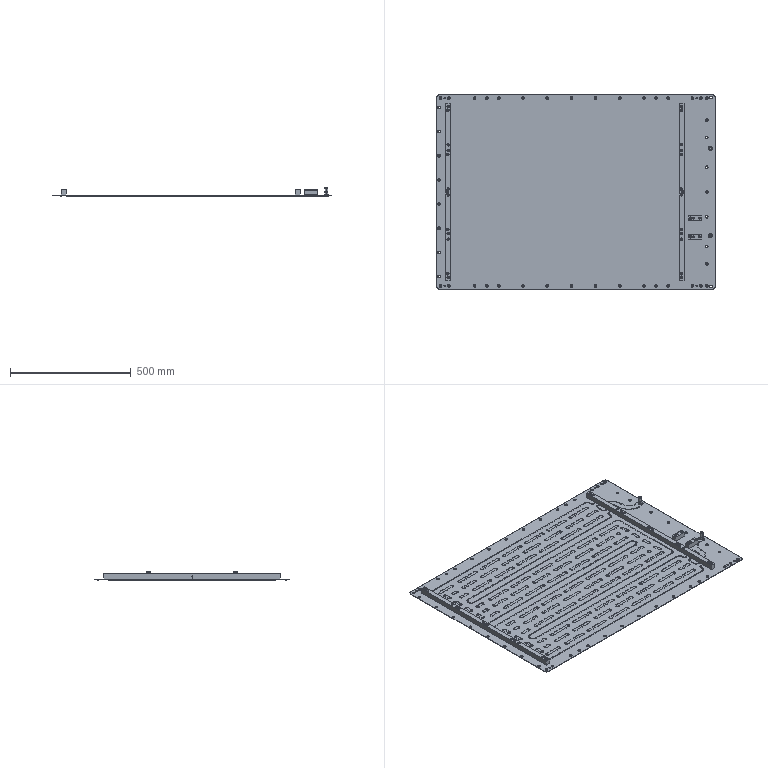Part | NX | features BREP 13 | 44 solids | 3714 faces | volume 2817494 mm3 | cylinder 1486 | torus 1245 | plane 678 | cone 212 | spline 93 | commonest cylinder face diameters 7 x352 5 x176 9 x176 6 x112 8 x110 8.5 x94